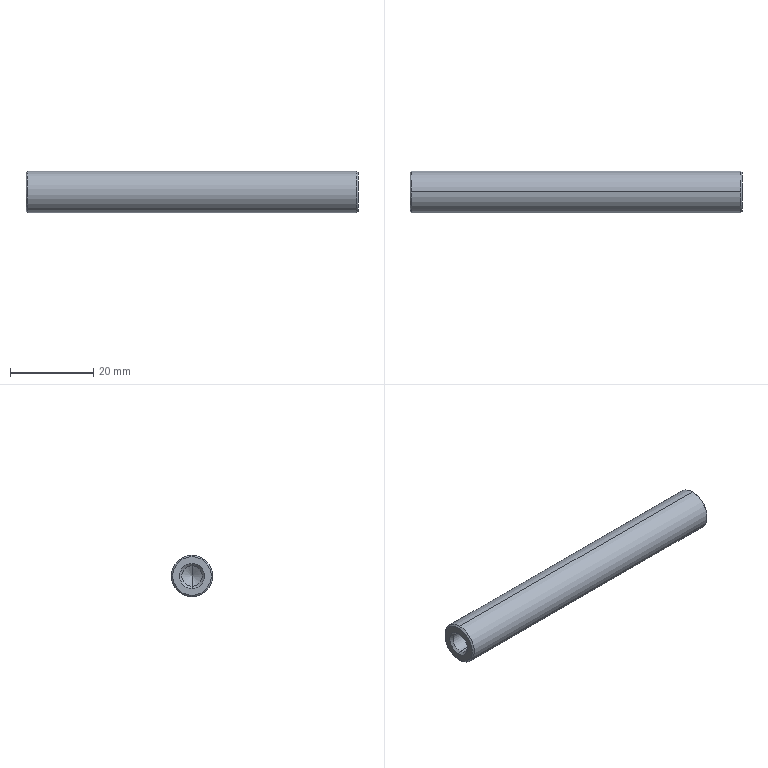Part | STEP file | SCD11-D10-L80-M6 | 1 solid | 14 faces | box 80 x 10 x 10 mm | volume 6034 mm3 | cone 8 | cylinder 4 | plane 2 | commonest cylinder face diameters 4.917 x2 10 x2
STEP:
#1=CARTESIAN_POINT('',(0.3536,0.,-5.));
#2=VERTEX_POINT('',#1);
#3=CARTESIAN_POINT('',(0.3536,0.,5.));
#4=VERTEX_POINT('',#3);
#5=CARTESIAN_POINT('',(0.3536,0.,0.));
#6=DIRECTION('',(1.,0.,0.));
#7=DIRECTION('',(0.,0.,-1.));
#8=AXIS2_PLACEMENT_3D('',#5,#6,#7);
#9=CIRCLE('',#8,5.);
#10=EDGE_CURVE('',#2,#4,#9,.T.);
#11=ORIENTED_EDGE('',*,*,#10,.T.);
#12=CARTESIAN_POINT('',(79.646,0.,5.));
#13=VERTEX_POINT('',#12);
#14=CARTESIAN_POINT('',(80.,0.,5.));
#15=DIRECTION('',(1.,0.,0.));
#16=VECTOR('',#15,1000.);
#17=LINE('',#14,#16);
#18=EDGE_CURVE('',#4,#13,#17,.T.);
#19=ORIENTED_EDGE('',*,*,#18,.T.);
#20=CARTESIAN_POINT('',(79.646,0.,-5.));
#21=VERTEX_POINT('',#20);
#22=CARTESIAN_POINT('',(79.646,0.,0.));
#23=DIRECTION('',(-1.,0.,0.));
#24=DIRECTION('',(0.,0.,-1.));
#25=AXIS2_PLACEMENT_3D('',#22,#23,#24);
#26=CIRCLE('',#25,5.);
#27=EDGE_CURVE('',#13,#21,#26,.T.);
#28=ORIENTED_EDGE('',*,*,#27,.T.);
#29=CARTESIAN_POINT('',(80.,0.,-5.));
#30=DIRECTION('',(1.,0.,0.));
#31=VECTOR('',#30,1000.);
#32=LINE('',#29,#31);
#33=EDGE_CURVE('',#2,#21,#32,.T.);
#34=ORIENTED_EDGE('',*,*,#33,.F.);
#35=EDGE_LOOP('',(#11,#19,#28,#34));
#36=FACE_OUTER_BOUND('',#35,.T.);
#37=CARTESIAN_POINT('',(80.,0.,0.));
#38=DIRECTION('',(1.,0.,0.));
#39=DIRECTION('',(0.,0.,-1.));
#40=AXIS2_PLACEMENT_3D('',#37,#38,#39);
#41=CYLINDRICAL_SURFACE('',#40,5.);
#42=ADVANCED_FACE('',(#36),#41,.T.);
#43=CARTESIAN_POINT('',(0.,0.,-4.646));
#44=VERTEX_POINT('',#43);
#45=CARTESIAN_POINT('',(0.,0.,4.646));
#46=VERTEX_POINT('',#45);
#47=CARTESIAN_POINT('',(0.,0.,0.));
#48=DIRECTION('',(1.,0.,0.));
#49=DIRECTION('',(0.,0.,-1.));
#50=AXIS2_PLACEMENT_3D('',#47,#48,#49);
#51=CIRCLE('',#50,4.646);
#52=EDGE_CURVE('',#44,#46,#51,.T.);
#53=ORIENTED_EDGE('',*,*,#52,.T.);
#54=CARTESIAN_POINT('',(0.3536,0.,5.));
#55=DIRECTION('',(0.7071,0.,0.7071));
#56=VECTOR('',#55,1000.);
#57=LINE('',#54,#56);
#58=EDGE_CURVE('',#46,#4,#57,.T.);
#59=ORIENTED_EDGE('',*,*,#58,.T.);
#60=ORIENTED_EDGE('',*,*,#10,.F.);
#61=CARTESIAN_POINT('',(0.3536,0.,-5.));
#62=DIRECTION('',(0.7071,0.,-0.7071));
#63=VECTOR('',#62,1000.);
#64=LINE('',#61,#63);
#65=EDGE_CURVE('',#44,#2,#64,.T.);
#66=ORIENTED_EDGE('',*,*,#65,.F.);
#67=EDGE_LOOP('',(#53,#59,#60,#66));
#68=FACE_OUTER_BOUND('',#67,.T.);
#69=CARTESIAN_POINT('',(0.3536,0.,0.));
#70=DIRECTION('',(1.,0.,0.));
#71=DIRECTION('',(0.,0.,-1.));
#72=AXIS2_PLACEMENT_3D('',#69,#70,#71);
#73=CONICAL_SURFACE('',#72,5.,0.7854);
#74=ADVANCED_FACE('',(#68),#73,.T.);
#75=CARTESIAN_POINT('',(80.,0.,4.646));
#76=VERTEX_POINT('',#75);
#77=CARTESIAN_POINT('',(80.,0.,-4.646));
#78=VERTEX_POINT('',#77);
#79=CARTESIAN_POINT('',(80.,0.,0.));
#80=DIRECTION('',(-1.,0.,0.));
#81=DIRECTION('',(0.,0.,1.));
#82=AXIS2_PLACEMENT_3D('',#79,#80,#81);
#83=CIRCLE('',#82,4.646);
#84=EDGE_CURVE('',#76,#78,#83,.T.);
#85=ORIENTED_EDGE('',*,*,#84,.T.);
#86=CARTESIAN_POINT('',(79.646,0.,-5.));
#87=DIRECTION('',(-0.7071,0.,-0.7071));
#88=VECTOR('',#87,1000.);
#89=LINE('',#86,#88);
#90=EDGE_CURVE('',#78,#21,#89,.T.);
#91=ORIENTED_EDGE('',*,*,#90,.T.);
#92=ORIENTED_EDGE('',*,*,#27,.F.);
#93=CARTESIAN_POINT('',(79.646,0.,5.));
#94=DIRECTION('',(-0.7071,0.,0.7071));
#95=VECTOR('',#94,1000.);
#96=LINE('',#93,#95);
#97=EDGE_CURVE('',#76,#13,#96,.T.);
#98=ORIENTED_EDGE('',*,*,#97,.F.);
#99=EDGE_LOOP('',(#85,#91,#92,#98));
#100=FACE_OUTER_BOUND('',#99,.T.);
#101=CARTESIAN_POINT('',(79.646,0.,0.));
#102=DIRECTION('',(-1.,0.,0.));
#103=DIRECTION('',(0.,0.,1.));
#104=AXIS2_PLACEMENT_3D('',#101,#102,#103);
#105=CONICAL_SURFACE('',#104,5.,0.7854);
#106=ADVANCED_FACE('',(#100),#105,.T.);
#107=CARTESIAN_POINT('',(0.5415,0.,-2.458));
#108=VERTEX_POINT('',#107);
#109=CARTESIAN_POINT('',(0.5415,0.,2.458));
#110=VERTEX_POINT('',#109);
#111=CARTESIAN_POINT('',(0.5415,0.,0.));
#112=DIRECTION('',(-1.,0.,0.));
#113=DIRECTION('',(0.,0.,1.));
#114=AXIS2_PLACEMENT_3D('',#111,#112,#113);
#115=CIRCLE('',#114,2.458);
#116=EDGE_CURVE('',#108,#110,#115,.T.);
#117=ORIENTED_EDGE('',*,*,#116,.F.);
#118=CARTESIAN_POINT('',(0.,0.,-3.));
#119=VERTEX_POINT('',#118);
#120=CARTESIAN_POINT('',(0.,0.,-3.));
#121=DIRECTION('',(-0.7071,0.,-0.7071));
#122=VECTOR('',#121,1000.);
#123=LINE('',#120,#122);
#124=EDGE_CURVE('',#108,#119,#123,.T.);
#125=ORIENTED_EDGE('',*,*,#124,.T.);
#126=CARTESIAN_POINT('',(0.,0.,3.));
#127=VERTEX_POINT('',#126);
#128=CARTESIAN_POINT('',(0.,0.,0.));
#129=DIRECTION('',(-1.,0.,0.));
#130=DIRECTION('',(0.,0.,1.));
#131=AXIS2_PLACEMENT_3D('',#128,#129,#130);
#132=CIRCLE('',#131,3.);
#133=EDGE_CURVE('',#119,#127,#132,.T.);
#134=ORIENTED_EDGE('',*,*,#133,.T.);
#135=CARTESIAN_POINT('',(0.,0.,3.));
#136=DIRECTION('',(-0.7071,0.,0.7071));
#137=VECTOR('',#136,1000.);
#138=LINE('',#135,#137);
#139=EDGE_CURVE('',#110,#127,#138,.T.);
#140=ORIENTED_EDGE('',*,*,#139,.F.);
#141=EDGE_LOOP('',(#117,#125,#134,#140));
#142=FACE_OUTER_BOUND('',#141,.T.);
#143=CARTESIAN_POINT('',(0.,0.,0.));
#144=DIRECTION('',(-1.,0.,0.));
#145=DIRECTION('',(0.,0.,1.));
#146=AXIS2_PLACEMENT_3D('',#143,#144,#145);
#147=CONICAL_SURFACE('',#146,3.,0.7854);
#148=ADVANCED_FACE('',(#142),#147,.F.);
#149=ORIENTED_EDGE('',*,*,#116,.T.);
#150=CARTESIAN_POINT('',(12.325,0.,2.458));
#151=VERTEX_POINT('',#150);
#152=CARTESIAN_POINT('',(80.,0.,2.459));
#153=DIRECTION('',(1.,0.,0.));
#154=VECTOR('',#153,1000.);
#155=LINE('',#152,#154);
#156=EDGE_CURVE('',#110,#151,#155,.T.);
#157=ORIENTED_EDGE('',*,*,#156,.T.);
#158=CARTESIAN_POINT('',(12.325,0.,-2.458));
#159=VERTEX_POINT('',#158);
#160=CARTESIAN_POINT('',(12.325,0.,0.));
#161=DIRECTION('',(-1.,0.,0.));
#162=DIRECTION('',(0.,0.,-1.));
#163=AXIS2_PLACEMENT_3D('',#160,#161,#162);
#164=CIRCLE('',#163,2.459);
#165=EDGE_CURVE('',#159,#151,#164,.T.);
#166=ORIENTED_EDGE('',*,*,#165,.F.);
#167=CARTESIAN_POINT('',(80.,0.,-2.459));
#168=DIRECTION('',(1.,0.,0.));
#169=VECTOR('',#168,1000.);
#170=LINE('',#167,#169);
#171=EDGE_CURVE('',#108,#159,#170,.T.);
#172=ORIENTED_EDGE('',*,*,#171,.F.);
#173=EDGE_LOOP('',(#149,#157,#166,#172));
#174=FACE_OUTER_BOUND('',#173,.T.);
#175=CARTESIAN_POINT('',(80.,0.,0.));
#176=DIRECTION('',(1.,0.,0.));
#177=DIRECTION('',(0.,0.,-1.));
#178=AXIS2_PLACEMENT_3D('',#175,#176,#177);
#179=CYLINDRICAL_SURFACE('',#178,2.459);
#180=ADVANCED_FACE('',(#174),#179,.F.);
#181=CARTESIAN_POINT('',(13.803,0.,0.));
#182=VERTEX_POINT('',#181);
#183=CARTESIAN_POINT('',(12.325,0.,2.458));
#184=DIRECTION('',(-0.515,0.,0.8572));
#185=VECTOR('',#184,1000.);
#186=LINE('',#183,#185);
#187=EDGE_CURVE('',#182,#151,#186,.T.);
#188=ORIENTED_EDGE('',*,*,#187,.F.);
#189=CARTESIAN_POINT('',(12.325,0.,-2.458));
#190=DIRECTION('',(-0.515,0.,-0.8572));
#191=VECTOR('',#190,1000.);
#192=LINE('',#189,#191);
#193=EDGE_CURVE('',#182,#159,#192,.T.);
#194=ORIENTED_EDGE('',*,*,#193,.T.);
#195=ORIENTED_EDGE('',*,*,#165,.T.);
#196=EDGE_LOOP('',(#188,#194,#195));
#197=FACE_OUTER_BOUND('',#196,.T.);
#198=CARTESIAN_POINT('',(12.325,0.,0.));
#199=DIRECTION('',(-1.,0.,0.));
#200=DIRECTION('',(0.,0.,1.));
#201=AXIS2_PLACEMENT_3D('',#198,#199,#200);
#202=CONICAL_SURFACE('',#201,2.458,1.03);
#203=ADVANCED_FACE('',(#197),#202,.F.);
#204=ORIENTED_EDGE('',*,*,#18,.F.);
#205=CARTESIAN_POINT('',(0.3536,0.,0.));
#206=DIRECTION('',(1.,0.,0.));
#207=DIRECTION('',(0.,0.,-1.));
#208=AXIS2_PLACEMENT_3D('',#205,#206,#207);
#209=CIRCLE('',#208,5.);
#210=EDGE_CURVE('',#4,#2,#209,.T.);
#211=ORIENTED_EDGE('',*,*,#210,.T.);
#212=ORIENTED_EDGE('',*,*,#33,.T.);
#213=CARTESIAN_POINT('',(79.646,0.,0.));
#214=DIRECTION('',(-1.,0.,0.));
#215=DIRECTION('',(0.,0.,-1.));
#216=AXIS2_PLACEMENT_3D('',#213,#214,#215);
#217=CIRCLE('',#216,5.);
#218=EDGE_CURVE('',#21,#13,#217,.T.);
#219=ORIENTED_EDGE('',*,*,#218,.T.);
#220=EDGE_LOOP('',(#204,#211,#212,#219));
#221=FACE_OUTER_BOUND('',#220,.T.);
#222=CARTESIAN_POINT('',(80.,0.,0.));
#223=DIRECTION('',(1.,0.,0.));
#224=DIRECTION('',(0.,0.,-1.));
#225=AXIS2_PLACEMENT_3D('',#222,#223,#224);
#226=CYLINDRICAL_SURFACE('',#225,5.);
#227=ADVANCED_FACE('',(#221),#226,.T.);
#228=ORIENTED_EDGE('',*,*,#58,.F.);
#229=CARTESIAN_POINT('',(0.,0.,0.));
#230=DIRECTION('',(1.,0.,0.));
#231=DIRECTION('',(0.,0.,-1.));
#232=AXIS2_PLACEMENT_3D('',#229,#230,#231);
#233=CIRCLE('',#232,4.646);
#234=EDGE_CURVE('',#46,#44,#233,.T.);
#235=ORIENTED_EDGE('',*,*,#234,.T.);
#236=ORIENTED_EDGE('',*,*,#65,.T.);
#237=ORIENTED_EDGE('',*,*,#210,.F.);
#238=EDGE_LOOP('',(#228,#235,#236,#237));
#239=FACE_OUTER_BOUND('',#238,.T.);
#240=CARTESIAN_POINT('',(0.3536,0.,0.));
#241=DIRECTION('',(1.,0.,0.));
#242=DIRECTION('',(0.,0.,-1.));
#243=AXIS2_PLACEMENT_3D('',#240,#241,#242);
#244=CONICAL_SURFACE('',#243,5.,0.7854);
#245=ADVANCED_FACE('',(#239),#244,.T.);
#246=ORIENTED_EDGE('',*,*,#90,.F.);
#247=CARTESIAN_POINT('',(80.,0.,0.));
#248=DIRECTION('',(-1.,0.,0.));
#249=DIRECTION('',(0.,0.,1.));
#250=AXIS2_PLACEMENT_3D('',#247,#248,#249);
#251=CIRCLE('',#250,4.646);
#252=EDGE_CURVE('',#78,#76,#251,.T.);
#253=ORIENTED_EDGE('',*,*,#252,.T.);
#254=ORIENTED_EDGE('',*,*,#97,.T.);
#255=ORIENTED_EDGE('',*,*,#218,.F.);
#256=EDGE_LOOP('',(#246,#253,#254,#255));
#257=FACE_OUTER_BOUND('',#256,.T.);
#258=CARTESIAN_POINT('',(79.646,0.,0.));
#259=DIRECTION('',(-1.,0.,0.));
#260=DIRECTION('',(0.,0.,1.));
#261=AXIS2_PLACEMENT_3D('',#258,#259,#260);
#262=CONICAL_SURFACE('',#261,5.,0.7854);
#263=ADVANCED_FACE('',(#257),#262,.T.);
#264=CARTESIAN_POINT('',(0.,0.,0.));
#265=DIRECTION('',(-1.,0.,0.));
#266=DIRECTION('',(0.,0.,1.));
#267=AXIS2_PLACEMENT_3D('',#264,#265,#266);
#268=CIRCLE('',#267,3.);
#269=EDGE_CURVE('',#127,#119,#268,.T.);
#270=ORIENTED_EDGE('',*,*,#269,.F.);
#271=ORIENTED_EDGE('',*,*,#133,.F.);
#272=EDGE_LOOP('',(#270,#271));
#273=FACE_BOUND('',#272,.T.);
#274=ORIENTED_EDGE('',*,*,#52,.F.);
#275=ORIENTED_EDGE('',*,*,#234,.F.);
#276=EDGE_LOOP('',(#274,#275));
#277=FACE_OUTER_BOUND('',#276,.T.);
#278=CARTESIAN_POINT('',(0.,3.,0.));
#279=DIRECTION('',(1.,0.,0.));
#280=DIRECTION('',(0.,0.,-1.));
#281=AXIS2_PLACEMENT_3D('',#278,#279,#280);
#282=PLANE('',#281);
#283=ADVANCED_FACE('',(#273,#277),#282,.F.);
#284=ORIENTED_EDGE('',*,*,#84,.F.);
#285=ORIENTED_EDGE('',*,*,#252,.F.);
#286=EDGE_LOOP('',(#284,#285));
#287=FACE_OUTER_BOUND('',#286,.T.);
#288=CARTESIAN_POINT('',(80.,4.646,0.));
#289=DIRECTION('',(-1.,0.,0.));
#290=DIRECTION('',(0.,0.,1.));
#291=AXIS2_PLACEMENT_3D('',#288,#289,#290);
#292=PLANE('',#291);
#293=ADVANCED_FACE('',(#287),#292,.F.);
#294=ORIENTED_EDGE('',*,*,#124,.F.);
#295=CARTESIAN_POINT('',(0.5415,0.,0.));
#296=DIRECTION('',(-1.,0.,0.));
#297=DIRECTION('',(0.,0.,1.));
#298=AXIS2_PLACEMENT_3D('',#295,#296,#297);
#299=CIRCLE('',#298,2.458);
#300=EDGE_CURVE('',#110,#108,#299,.T.);
#301=ORIENTED_EDGE('',*,*,#300,.F.);
#302=ORIENTED_EDGE('',*,*,#139,.T.);
#303=ORIENTED_EDGE('',*,*,#269,.T.);
#304=EDGE_LOOP('',(#294,#301,#302,#303));
#305=FACE_OUTER_BOUND('',#304,.T.);
#306=CARTESIAN_POINT('',(0.,0.,0.));
#307=DIRECTION('',(-1.,0.,0.));
#308=DIRECTION('',(0.,0.,1.));
#309=AXIS2_PLACEMENT_3D('',#306,#307,#308);
#310=CONICAL_SURFACE('',#309,3.,0.7854);
#311=ADVANCED_FACE('',(#305),#310,.F.);
#312=ORIENTED_EDGE('',*,*,#156,.F.);
#313=ORIENTED_EDGE('',*,*,#300,.T.);
#314=ORIENTED_EDGE('',*,*,#171,.T.);
#315=CARTESIAN_POINT('',(12.325,0.,0.));
#316=DIRECTION('',(-1.,0.,0.));
#317=DIRECTION('',(0.,0.,-1.));
#318=AXIS2_PLACEMENT_3D('',#315,#316,#317);
#319=CIRCLE('',#318,2.459);
#320=EDGE_CURVE('',#151,#159,#319,.T.);
#321=ORIENTED_EDGE('',*,*,#320,.F.);
#322=EDGE_LOOP('',(#312,#313,#314,#321));
#323=FACE_OUTER_BOUND('',#322,.T.);
#324=CARTESIAN_POINT('',(80.,0.,0.));
#325=DIRECTION('',(1.,0.,0.));
#326=DIRECTION('',(0.,0.,-1.));
#327=AXIS2_PLACEMENT_3D('',#324,#325,#326);
#328=CYLINDRICAL_SURFACE('',#327,2.459);
#329=ADVANCED_FACE('',(#323),#328,.F.);
#330=ORIENTED_EDGE('',*,*,#193,.F.);
#331=ORIENTED_EDGE('',*,*,#187,.T.);
#332=ORIENTED_EDGE('',*,*,#320,.T.);
#333=EDGE_LOOP('',(#330,#331,#332));
#334=FACE_OUTER_BOUND('',#333,.T.);
#335=CARTESIAN_POINT('',(12.325,0.,0.));
#336=DIRECTION('',(-1.,0.,0.));
#337=DIRECTION('',(0.,0.,1.));
#338=AXIS2_PLACEMENT_3D('',#335,#336,#337);
#339=CONICAL_SURFACE('',#338,2.458,1.03);
#340=ADVANCED_FACE('',(#334),#339,.F.);
#341=CLOSED_SHELL('',(#42,#74,#106,#148,#180,#203,#227,#245,#263,#283,#293,#311,#329,#340));
#342=MANIFOLD_SOLID_BREP('',#341);
#343=CARTESIAN_POINT('',(0.,0.,0.));
#344=DIRECTION('',(0.,0.,1.));
#345=DIRECTION('',(1.,0.,0.));
#346=AXIS2_PLACEMENT_3D('',#343,#344,#345);
#347=(LENGTH_UNIT()NAMED_UNIT(*)SI_UNIT(.MILLI.,.METRE.));
#348=UNCERTAINTY_MEASURE_WITH_UNIT(LENGTH_MEASURE(0.00001),#347,'','');
#349=(NAMED_UNIT(*)PLANE_ANGLE_UNIT()SI_UNIT($,.RADIAN.));
#350=(NAMED_UNIT(*)SI_UNIT($,.STERADIAN.)SOLID_ANGLE_UNIT());
#351=(GEOMETRIC_REPRESENTATION_CONTEXT(3)GLOBAL_UNCERTAINTY_ASSIGNED_CONTEXT((#348))GLOBAL_UNIT_ASSIGNED_CONTEXT((#347,#349,#350))REPRESENTATION_CONTEXT('',''));
#352=ADVANCED_BREP_SHAPE_REPRESENTATION('',(#342,#346),#351);